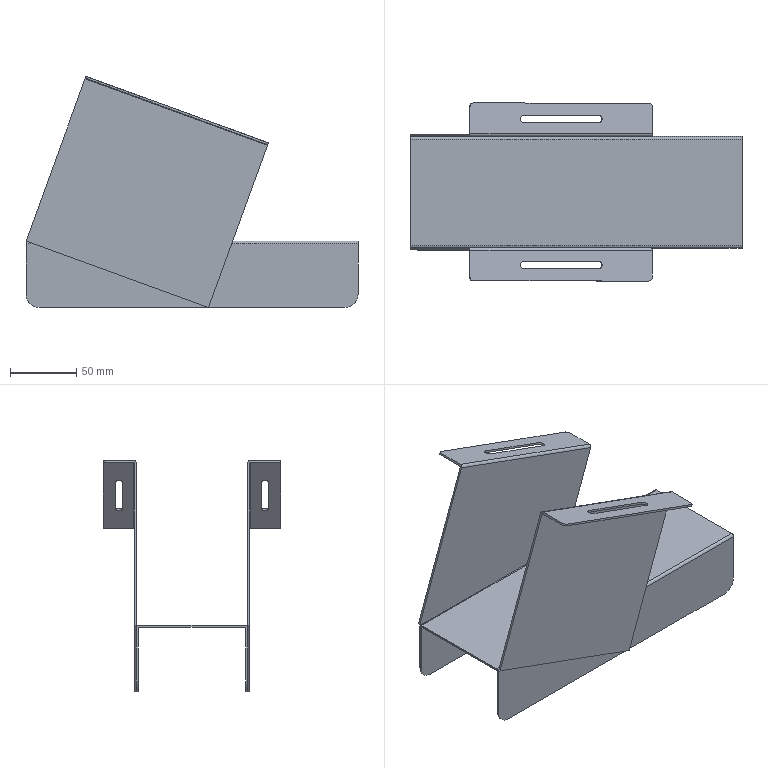Part | SolidWorks | features BaseBody 3 | 3 solids | 68 faces | box 250 x 134 x 174.039 mm | volume 134233 mm3 | plane 46 | cylinder 22 | commonest cylinder face diameters 5.5 x6 1 x4 4 x4 6 x4 20 x4